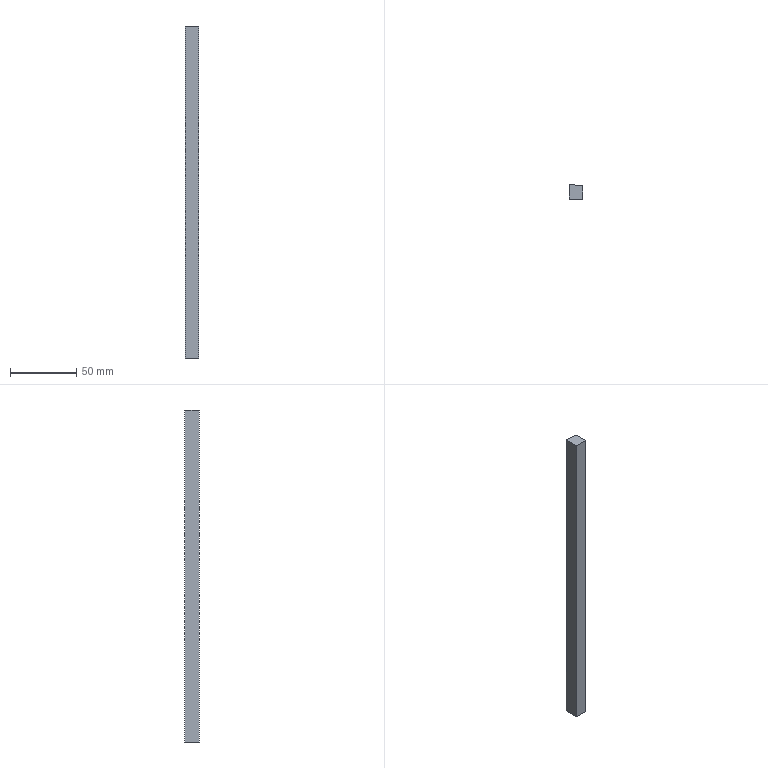Part | SolidWorks | features Extrusion 1 | 1 solid | 6 faces | box 10 x 11.228 x 250 mm | volume 26535 mm3 | plane 6
STEP:
#1=CARTESIAN_POINT('',(0.,0.,0.));
#2=VERTEX_POINT('',#1);
#3=CARTESIAN_POINT('',(10.,0.,0.));
#4=VERTEX_POINT('',#3);
#5=CARTESIAN_POINT('',(0.,0.,0.));
#6=DIRECTION('',(1.,0.,0.));
#7=VECTOR('',#6,1000.);
#8=LINE('',#5,#7);
#9=EDGE_CURVE('',#2,#4,#8,.T.);
#10=ORIENTED_EDGE('',*,*,#9,.T.);
#11=CARTESIAN_POINT('',(10.,0.,250.));
#12=VERTEX_POINT('',#11);
#13=CARTESIAN_POINT('',(10.,0.,250.));
#14=DIRECTION('',(0.,0.,-1.));
#15=VECTOR('',#14,1000.);
#16=LINE('',#13,#15);
#17=EDGE_CURVE('',#12,#4,#16,.T.);
#18=ORIENTED_EDGE('',*,*,#17,.F.);
#19=CARTESIAN_POINT('',(0.,0.,250.));
#20=VERTEX_POINT('',#19);
#21=CARTESIAN_POINT('',(0.,0.,250.));
#22=DIRECTION('',(1.,0.,0.));
#23=VECTOR('',#22,1000.);
#24=LINE('',#21,#23);
#25=EDGE_CURVE('',#20,#12,#24,.T.);
#26=ORIENTED_EDGE('',*,*,#25,.F.);
#27=CARTESIAN_POINT('',(0.,0.,250.));
#28=DIRECTION('',(0.,0.,-1.));
#29=VECTOR('',#28,1000.);
#30=LINE('',#27,#29);
#31=EDGE_CURVE('',#20,#2,#30,.T.);
#32=ORIENTED_EDGE('',*,*,#31,.T.);
#33=EDGE_LOOP('',(#10,#18,#26,#32));
#34=FACE_OUTER_BOUND('',#33,.T.);
#35=CARTESIAN_POINT('',(0.,0.,250.));
#36=DIRECTION('',(0.,1.,0.));
#37=DIRECTION('',(0.,0.,1.));
#38=AXIS2_PLACEMENT_3D('',#35,#36,#37);
#39=PLANE('',#38);
#40=ADVANCED_FACE('',(#34),#39,.F.);
#41=CARTESIAN_POINT('',(10.,10.,0.));
#42=VERTEX_POINT('',#41);
#43=CARTESIAN_POINT('',(10.,0.,0.));
#44=DIRECTION('',(0.,1.,0.));
#45=VECTOR('',#44,1000.);
#46=LINE('',#43,#45);
#47=EDGE_CURVE('',#4,#42,#46,.T.);
#48=ORIENTED_EDGE('',*,*,#47,.T.);
#49=CARTESIAN_POINT('',(10.,10.,250.));
#50=VERTEX_POINT('',#49);
#51=CARTESIAN_POINT('',(10.,10.,250.));
#52=DIRECTION('',(0.,0.,-1.));
#53=VECTOR('',#52,1000.);
#54=LINE('',#51,#53);
#55=EDGE_CURVE('',#50,#42,#54,.T.);
#56=ORIENTED_EDGE('',*,*,#55,.F.);
#57=CARTESIAN_POINT('',(10.,0.,250.));
#58=DIRECTION('',(0.,1.,0.));
#59=VECTOR('',#58,1000.);
#60=LINE('',#57,#59);
#61=EDGE_CURVE('',#12,#50,#60,.T.);
#62=ORIENTED_EDGE('',*,*,#61,.F.);
#63=ORIENTED_EDGE('',*,*,#17,.T.);
#64=EDGE_LOOP('',(#48,#56,#62,#63));
#65=FACE_OUTER_BOUND('',#64,.T.);
#66=CARTESIAN_POINT('',(10.,0.,250.));
#67=DIRECTION('',(-1.,0.,0.));
#68=DIRECTION('',(0.,0.,1.));
#69=AXIS2_PLACEMENT_3D('',#66,#67,#68);
#70=PLANE('',#69);
#71=ADVANCED_FACE('',(#65),#70,.F.);
#72=CARTESIAN_POINT('',(0.,11.228,0.));
#73=VERTEX_POINT('',#72);
#74=CARTESIAN_POINT('',(10.,10.,0.));
#75=DIRECTION('',(-0.9925,0.1219,0.));
#76=VECTOR('',#75,1000.);
#77=LINE('',#74,#76);
#78=EDGE_CURVE('',#42,#73,#77,.T.);
#79=ORIENTED_EDGE('',*,*,#78,.T.);
#80=CARTESIAN_POINT('',(0.,11.228,250.));
#81=VERTEX_POINT('',#80);
#82=CARTESIAN_POINT('',(0.,11.228,250.));
#83=DIRECTION('',(0.,0.,-1.));
#84=VECTOR('',#83,1000.);
#85=LINE('',#82,#84);
#86=EDGE_CURVE('',#81,#73,#85,.T.);
#87=ORIENTED_EDGE('',*,*,#86,.F.);
#88=CARTESIAN_POINT('',(10.,10.,250.));
#89=DIRECTION('',(-0.9925,0.1219,0.));
#90=VECTOR('',#89,1000.);
#91=LINE('',#88,#90);
#92=EDGE_CURVE('',#50,#81,#91,.T.);
#93=ORIENTED_EDGE('',*,*,#92,.F.);
#94=ORIENTED_EDGE('',*,*,#55,.T.);
#95=EDGE_LOOP('',(#79,#87,#93,#94));
#96=FACE_OUTER_BOUND('',#95,.T.);
#97=CARTESIAN_POINT('',(10.,10.,250.));
#98=DIRECTION('',(-0.1219,-0.9925,0.));
#99=DIRECTION('',(0.9925,-0.1219,0.));
#100=AXIS2_PLACEMENT_3D('',#97,#98,#99);
#101=PLANE('',#100);
#102=ADVANCED_FACE('',(#96),#101,.F.);
#103=CARTESIAN_POINT('',(0.,0.,0.));
#104=DIRECTION('',(0.,-1.,0.));
#105=VECTOR('',#104,1000.);
#106=LINE('',#103,#105);
#107=EDGE_CURVE('',#73,#2,#106,.T.);
#108=ORIENTED_EDGE('',*,*,#107,.T.);
#109=ORIENTED_EDGE('',*,*,#31,.F.);
#110=CARTESIAN_POINT('',(0.,0.,250.));
#111=DIRECTION('',(0.,-1.,0.));
#112=VECTOR('',#111,1000.);
#113=LINE('',#110,#112);
#114=EDGE_CURVE('',#81,#20,#113,.T.);
#115=ORIENTED_EDGE('',*,*,#114,.F.);
#116=ORIENTED_EDGE('',*,*,#86,.T.);
#117=EDGE_LOOP('',(#108,#109,#115,#116));
#118=FACE_OUTER_BOUND('',#117,.T.);
#119=CARTESIAN_POINT('',(0.,0.,250.));
#120=DIRECTION('',(1.,0.,0.));
#121=DIRECTION('',(0.,0.,-1.));
#122=AXIS2_PLACEMENT_3D('',#119,#120,#121);
#123=PLANE('',#122);
#124=ADVANCED_FACE('',(#118),#123,.F.);
#125=ORIENTED_EDGE('',*,*,#25,.T.);
#126=ORIENTED_EDGE('',*,*,#61,.T.);
#127=ORIENTED_EDGE('',*,*,#92,.T.);
#128=ORIENTED_EDGE('',*,*,#114,.T.);
#129=EDGE_LOOP('',(#125,#126,#127,#128));
#130=FACE_OUTER_BOUND('',#129,.T.);
#131=CARTESIAN_POINT('',(0.,0.,250.));
#132=DIRECTION('',(0.,0.,1.));
#133=DIRECTION('',(1.,0.,0.));
#134=AXIS2_PLACEMENT_3D('',#131,#132,#133);
#135=PLANE('',#134);
#136=ADVANCED_FACE('',(#130),#135,.T.);
#137=ORIENTED_EDGE('',*,*,#9,.F.);
#138=ORIENTED_EDGE('',*,*,#107,.F.);
#139=ORIENTED_EDGE('',*,*,#78,.F.);
#140=ORIENTED_EDGE('',*,*,#47,.F.);
#141=EDGE_LOOP('',(#137,#138,#139,#140));
#142=FACE_OUTER_BOUND('',#141,.T.);
#143=CARTESIAN_POINT('',(0.,0.,0.));
#144=DIRECTION('',(0.,0.,1.));
#145=DIRECTION('',(1.,0.,0.));
#146=AXIS2_PLACEMENT_3D('',#143,#144,#145);
#147=PLANE('',#146);
#148=ADVANCED_FACE('',(#142),#147,.F.);
#149=CLOSED_SHELL('',(#40,#71,#102,#124,#136,#148));
#150=MANIFOLD_SOLID_BREP('',#149);
#151=CARTESIAN_POINT('',(0.,0.,0.));
#152=DIRECTION('',(0.,0.,1.));
#153=DIRECTION('',(1.,0.,0.));
#154=AXIS2_PLACEMENT_3D('',#151,#152,#153);
#155=(LENGTH_UNIT()NAMED_UNIT(*)SI_UNIT(.MILLI.,.METRE.));
#156=UNCERTAINTY_MEASURE_WITH_UNIT(LENGTH_MEASURE(0.00001),#155,'','');
#157=(NAMED_UNIT(*)PLANE_ANGLE_UNIT()SI_UNIT($,.RADIAN.));
#158=(NAMED_UNIT(*)SI_UNIT($,.STERADIAN.)SOLID_ANGLE_UNIT());
#159=(GEOMETRIC_REPRESENTATION_CONTEXT(3)GLOBAL_UNCERTAINTY_ASSIGNED_CONTEXT((#156))GLOBAL_UNIT_ASSIGNED_CONTEXT((#155,#157,#158))REPRESENTATION_CONTEXT('',''));
#160=ADVANCED_BREP_SHAPE_REPRESENTATION('',(#150,#154),#159);